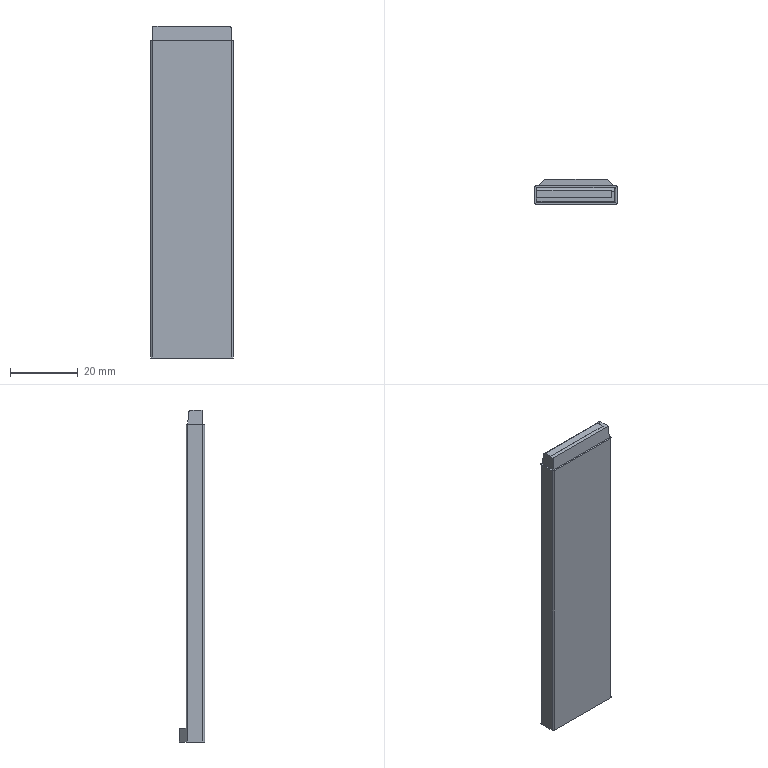Part | Creo | 1 solid | 23 faces | box 24.5 x 7.5 x 98.362 mm | volume 13240 mm3 | plane 18 | cylinder 5 | commonest cylinder face diameters 1 x4 2.01 x1
STEP:
#1=CARTESIAN_POINT('',(0.,0.,0.));
#2=DIRECTION('',(0.,0.,1.));
#3=DIRECTION('',(1.,0.,0.));
#4=AXIS2_PLACEMENT_3D('',#1,#2,#3);
#5=CARTESIAN_POINT('',(-40.598,53.591,40.081));
#6=VERTEX_POINT('',#5);
#7=CARTESIAN_POINT('',(-40.598,53.591,-54.09));
#8=VERTEX_POINT('',#7);
#9=CARTESIAN_POINT('',(-40.598,53.591,40.081));
#10=DIRECTION('',(0.,0.,-1.));
#11=VECTOR('',#10,94.171);
#12=LINE('',#9,#11);
#13=EDGE_CURVE('',#6,#8,#12,.T.);
#14=ORIENTED_EDGE('',*,*,#13,.T.);
#15=CARTESIAN_POINT('',(-40.598,58.091,-54.09));
#16=VERTEX_POINT('',#15);
#17=CARTESIAN_POINT('',(-40.598,53.591,-54.09));
#18=DIRECTION('',(0.,1.,0.));
#19=VECTOR('',#18,4.5);
#20=LINE('',#17,#19);
#21=EDGE_CURVE('',#8,#16,#20,.T.);
#22=ORIENTED_EDGE('',*,*,#21,.T.);
#23=CARTESIAN_POINT('',(-40.598,58.091,40.081));
#24=VERTEX_POINT('',#23);
#25=CARTESIAN_POINT('',(-40.598,58.091,-54.09));
#26=DIRECTION('',(0.,0.,1.));
#27=VECTOR('',#26,94.171);
#28=LINE('',#25,#27);
#29=EDGE_CURVE('',#16,#24,#28,.T.);
#30=ORIENTED_EDGE('',*,*,#29,.T.);
#31=CARTESIAN_POINT('',(-40.598,58.091,40.081));
#32=DIRECTION('',(0.,-1.,0.));
#33=VECTOR('',#32,4.5);
#34=LINE('',#31,#33);
#35=EDGE_CURVE('',#24,#6,#34,.T.);
#36=ORIENTED_EDGE('',*,*,#35,.T.);
#37=EDGE_LOOP('',(#14,#22,#30,#36));
#38=FACE_OUTER_BOUND('',#37,.F.);
#39=CARTESIAN_POINT('',(-40.598,58.591,68.91));
#40=DIRECTION('',(1.,0.,0.));
#41=DIRECTION('',(0.,0.,-1.));
#42=AXIS2_PLACEMENT_3D('',#39,#40,#41);
#43=PLANE('',#42);
#44=ADVANCED_FACE('',(#38),#43,.F.);
#45=CARTESIAN_POINT('',(-40.098,53.091,40.081));
#46=VERTEX_POINT('',#45);
#47=CARTESIAN_POINT('',(-40.098,53.591,40.081));
#48=DIRECTION('',(0.,0.,1.));
#49=DIRECTION('',(-1.,0.,0.));
#50=AXIS2_PLACEMENT_3D('',#47,#48,#49);
#51=CIRCLE('',#50,0.5);
#52=EDGE_CURVE('',#6,#46,#51,.T.);
#53=ORIENTED_EDGE('',*,*,#52,.T.);
#54=CARTESIAN_POINT('',(-40.098,53.091,-54.09));
#55=VERTEX_POINT('',#54);
#56=CARTESIAN_POINT('',(-40.098,53.091,-54.09));
#57=DIRECTION('',(0.,0.,1.));
#58=VECTOR('',#57,94.171);
#59=LINE('',#56,#58);
#60=EDGE_CURVE('',#55,#46,#59,.T.);
#61=ORIENTED_EDGE('',*,*,#60,.F.);
#62=CARTESIAN_POINT('',(-40.098,53.591,-54.09));
#63=DIRECTION('',(0.,0.,-1.));
#64=DIRECTION('',(0.,-1.,0.));
#65=AXIS2_PLACEMENT_3D('',#62,#63,#64);
#66=CIRCLE('',#65,0.5);
#67=EDGE_CURVE('',#55,#8,#66,.T.);
#68=ORIENTED_EDGE('',*,*,#67,.T.);
#69=ORIENTED_EDGE('',*,*,#13,.F.);
#70=EDGE_LOOP('',(#53,#61,#68,#69));
#71=FACE_OUTER_BOUND('',#70,.F.);
#72=CARTESIAN_POINT('',(-40.098,53.591,68.91));
#73=DIRECTION('',(0.,0.,-1.));
#74=DIRECTION('',(-1.,0.,0.));
#75=AXIS2_PLACEMENT_3D('',#72,#73,#74);
#76=CYLINDRICAL_SURFACE('',#75,0.5);
#77=ADVANCED_FACE('',(#71),#76,.T.);
#78=CARTESIAN_POINT('',(-16.598,58.591,40.081));
#79=VERTEX_POINT('',#78);
#80=CARTESIAN_POINT('',(-40.098,58.591,40.081));
#81=VERTEX_POINT('',#80);
#82=CARTESIAN_POINT('',(-16.598,58.591,40.081));
#83=DIRECTION('',(-1.,0.,0.));
#84=VECTOR('',#83,23.5);
#85=LINE('',#82,#84);
#86=EDGE_CURVE('',#79,#81,#85,.T.);
#87=ORIENTED_EDGE('',*,*,#86,.F.);
#88=CARTESIAN_POINT('',(-16.098,58.091,40.081));
#89=VERTEX_POINT('',#88);
#90=CARTESIAN_POINT('',(-16.598,58.091,40.081));
#91=DIRECTION('',(0.,0.,1.));
#92=DIRECTION('',(1.,0.,0.));
#93=AXIS2_PLACEMENT_3D('',#90,#91,#92);
#94=CIRCLE('',#93,0.5);
#95=EDGE_CURVE('',#89,#79,#94,.T.);
#96=ORIENTED_EDGE('',*,*,#95,.F.);
#97=CARTESIAN_POINT('',(-16.098,53.591,40.081));
#98=VERTEX_POINT('',#97);
#99=CARTESIAN_POINT('',(-16.098,53.591,40.081));
#100=DIRECTION('',(0.,1.,0.));
#101=VECTOR('',#100,4.5);
#102=LINE('',#99,#101);
#103=EDGE_CURVE('',#98,#89,#102,.T.);
#104=ORIENTED_EDGE('',*,*,#103,.F.);
#105=CARTESIAN_POINT('',(-16.598,53.091,40.081));
#106=VERTEX_POINT('',#105);
#107=CARTESIAN_POINT('',(-16.598,53.591,40.081));
#108=DIRECTION('',(0.,0.,1.));
#109=DIRECTION('',(0.,-1.,0.));
#110=AXIS2_PLACEMENT_3D('',#107,#108,#109);
#111=CIRCLE('',#110,0.5);
#112=EDGE_CURVE('',#106,#98,#111,.T.);
#113=ORIENTED_EDGE('',*,*,#112,.F.);
#114=CARTESIAN_POINT('',(-40.098,53.091,40.081));
#115=DIRECTION('',(1.,0.,0.));
#116=VECTOR('',#115,23.5);
#117=LINE('',#114,#116);
#118=EDGE_CURVE('',#46,#106,#117,.T.);
#119=ORIENTED_EDGE('',*,*,#118,.F.);
#120=ORIENTED_EDGE('',*,*,#52,.F.);
#121=ORIENTED_EDGE('',*,*,#35,.F.);
#122=CARTESIAN_POINT('',(-40.098,58.091,40.081));
#123=DIRECTION('',(0.,0.,1.));
#124=DIRECTION('',(0.,1.,0.));
#125=AXIS2_PLACEMENT_3D('',#122,#123,#124);
#126=CIRCLE('',#125,0.5);
#127=EDGE_CURVE('',#81,#24,#126,.T.);
#128=ORIENTED_EDGE('',*,*,#127,.F.);
#129=EDGE_LOOP('',(#87,#96,#104,#113,#119,#120,#121,#128));
#130=FACE_OUTER_BOUND('',#129,.F.);
#131=CARTESIAN_POINT('',(-16.598,53.644,40.081));
#132=VERTEX_POINT('',#131);
#133=CARTESIAN_POINT('',(-40.14,53.644,40.081));
#134=VERTEX_POINT('',#133);
#135=CARTESIAN_POINT('',(-16.598,53.644,40.081));
#136=DIRECTION('',(-1.,0.,0.));
#137=VECTOR('',#136,23.542);
#138=LINE('',#135,#137);
#139=EDGE_CURVE('',#132,#134,#138,.T.);
#140=ORIENTED_EDGE('',*,*,#139,.F.);
#141=CARTESIAN_POINT('',(-16.598,58.091,40.081));
#142=VERTEX_POINT('',#141);
#143=CARTESIAN_POINT('',(-16.598,58.091,40.081));
#144=DIRECTION('',(-0.00000001,-1.,0.000000195));
#145=VECTOR('',#144,4.447);
#146=LINE('',#143,#145);
#147=EDGE_CURVE('',#142,#132,#146,.T.);
#148=ORIENTED_EDGE('',*,*,#147,.F.);
#149=CARTESIAN_POINT('',(-40.14,58.091,40.081));
#150=VERTEX_POINT('',#149);
#151=CARTESIAN_POINT('',(-16.598,58.091,40.081));
#152=DIRECTION('',(-1.,0.,0.));
#153=VECTOR('',#152,23.542);
#154=LINE('',#151,#153);
#155=EDGE_CURVE('',#142,#150,#154,.T.);
#156=ORIENTED_EDGE('',*,*,#155,.T.);
#157=CARTESIAN_POINT('',(-40.14,58.091,40.081));
#158=DIRECTION('',(0.00000001,-1.,0.000000195));
#159=VECTOR('',#158,4.447);
#160=LINE('',#157,#159);
#161=EDGE_CURVE('',#150,#134,#160,.T.);
#162=ORIENTED_EDGE('',*,*,#161,.T.);
#163=EDGE_LOOP('',(#140,#148,#156,#162));
#164=FACE_BOUND('',#163,.F.);
#165=CARTESIAN_POINT('',(-17.817,-88.35,40.081));
#166=DIRECTION('',(0.,0.,1.));
#167=DIRECTION('',(-1.,0.,0.));
#168=AXIS2_PLACEMENT_3D('',#165,#166,#167);
#169=PLANE('',#168);
#170=ADVANCED_FACE('',(#130,#164),#169,.T.);
#171=CARTESIAN_POINT('',(-40.098,58.591,-54.09));
#172=VERTEX_POINT('',#171);
#173=CARTESIAN_POINT('',(-40.098,58.591,40.081));
#174=DIRECTION('',(0.,0.,-1.));
#175=VECTOR('',#174,94.171);
#176=LINE('',#173,#175);
#177=EDGE_CURVE('',#81,#172,#176,.T.);
#178=ORIENTED_EDGE('',*,*,#177,.T.);
#179=CARTESIAN_POINT('',(-39.598,58.591,-54.09));
#180=VERTEX_POINT('',#179);
#181=CARTESIAN_POINT('',(-40.098,58.591,-54.09));
#182=DIRECTION('',(1.,0.,0.));
#183=VECTOR('',#182,0.5);
#184=LINE('',#181,#183);
#185=EDGE_CURVE('',#172,#180,#184,.T.);
#186=ORIENTED_EDGE('',*,*,#185,.T.);
#187=CARTESIAN_POINT('',(-39.598,58.591,-50.09));
#188=VERTEX_POINT('',#187);
#189=CARTESIAN_POINT('',(-39.598,58.591,-54.09));
#190=DIRECTION('',(0.,0.,1.));
#191=VECTOR('',#190,4.);
#192=LINE('',#189,#191);
#193=EDGE_CURVE('',#180,#188,#192,.T.);
#194=ORIENTED_EDGE('',*,*,#193,.T.);
#195=CARTESIAN_POINT('',(-17.098,58.591,-50.09));
#196=VERTEX_POINT('',#195);
#197=CARTESIAN_POINT('',(-39.598,58.591,-50.09));
#198=DIRECTION('',(1.,0.,0.));
#199=VECTOR('',#198,22.5);
#200=LINE('',#197,#199);
#201=EDGE_CURVE('',#188,#196,#200,.T.);
#202=ORIENTED_EDGE('',*,*,#201,.T.);
#203=CARTESIAN_POINT('',(-17.098,58.591,-54.09));
#204=VERTEX_POINT('',#203);
#205=CARTESIAN_POINT('',(-17.098,58.591,-50.09));
#206=DIRECTION('',(0.,0.,-1.));
#207=VECTOR('',#206,4.);
#208=LINE('',#205,#207);
#209=EDGE_CURVE('',#196,#204,#208,.T.);
#210=ORIENTED_EDGE('',*,*,#209,.T.);
#211=CARTESIAN_POINT('',(-16.598,58.591,-54.09));
#212=VERTEX_POINT('',#211);
#213=CARTESIAN_POINT('',(-17.098,58.591,-54.09));
#214=DIRECTION('',(1.,0.,0.));
#215=VECTOR('',#214,0.5);
#216=LINE('',#213,#215);
#217=EDGE_CURVE('',#204,#212,#216,.T.);
#218=ORIENTED_EDGE('',*,*,#217,.T.);
#219=CARTESIAN_POINT('',(-16.598,58.591,-54.09));
#220=DIRECTION('',(0.,0.,1.));
#221=VECTOR('',#220,94.171);
#222=LINE('',#219,#221);
#223=EDGE_CURVE('',#212,#79,#222,.T.);
#224=ORIENTED_EDGE('',*,*,#223,.T.);
#225=ORIENTED_EDGE('',*,*,#86,.T.);
#226=EDGE_LOOP('',(#178,#186,#194,#202,#210,#218,#224,#225));
#227=FACE_OUTER_BOUND('',#226,.F.);
#228=CARTESIAN_POINT('',(-16.098,58.591,68.91));
#229=DIRECTION('',(0.,-1.,0.));
#230=DIRECTION('',(0.,0.,-1.));
#231=AXIS2_PLACEMENT_3D('',#228,#229,#230);
#232=PLANE('',#231);
#233=ADVANCED_FACE('',(#227),#232,.F.);
#234=ORIENTED_EDGE('',*,*,#127,.T.);
#235=ORIENTED_EDGE('',*,*,#29,.F.);
#236=CARTESIAN_POINT('',(-40.098,58.091,-54.09));
#237=DIRECTION('',(0.,0.,-1.));
#238=DIRECTION('',(-1.,0.,0.));
#239=AXIS2_PLACEMENT_3D('',#236,#237,#238);
#240=CIRCLE('',#239,0.5);
#241=EDGE_CURVE('',#16,#172,#240,.T.);
#242=ORIENTED_EDGE('',*,*,#241,.T.);
#243=ORIENTED_EDGE('',*,*,#177,.F.);
#244=EDGE_LOOP('',(#234,#235,#242,#243));
#245=FACE_OUTER_BOUND('',#244,.F.);
#246=CARTESIAN_POINT('',(-40.098,58.091,68.91));
#247=DIRECTION('',(0.,0.,-1.));
#248=DIRECTION('',(-1.,0.,0.));
#249=AXIS2_PLACEMENT_3D('',#246,#247,#248);
#250=CYLINDRICAL_SURFACE('',#249,0.5);
#251=ADVANCED_FACE('',(#245),#250,.T.);
#252=CARTESIAN_POINT('',(-37.598,60.591,-54.09));
#253=VERTEX_POINT('',#252);
#254=CARTESIAN_POINT('',(-19.098,60.591,-54.09));
#255=VERTEX_POINT('',#254);
#256=CARTESIAN_POINT('',(-37.598,60.591,-54.09));
#257=DIRECTION('',(1.,0.,0.));
#258=VECTOR('',#257,18.5);
#259=LINE('',#256,#258);
#260=EDGE_CURVE('',#253,#255,#259,.T.);
#261=ORIENTED_EDGE('',*,*,#260,.F.);
#262=CARTESIAN_POINT('',(-39.598,58.591,-54.09));
#263=DIRECTION('',(0.7071,0.7071,0.));
#264=VECTOR('',#263,2.828);
#265=LINE('',#262,#264);
#266=EDGE_CURVE('',#180,#253,#265,.T.);
#267=ORIENTED_EDGE('',*,*,#266,.F.);
#268=ORIENTED_EDGE('',*,*,#185,.F.);
#269=ORIENTED_EDGE('',*,*,#241,.F.);
#270=ORIENTED_EDGE('',*,*,#21,.F.);
#271=ORIENTED_EDGE('',*,*,#67,.F.);
#272=CARTESIAN_POINT('',(-16.598,53.091,-54.09));
#273=VERTEX_POINT('',#272);
#274=CARTESIAN_POINT('',(-16.598,53.091,-54.09));
#275=DIRECTION('',(-1.,0.,0.));
#276=VECTOR('',#275,23.5);
#277=LINE('',#274,#276);
#278=EDGE_CURVE('',#273,#55,#277,.T.);
#279=ORIENTED_EDGE('',*,*,#278,.F.);
#280=CARTESIAN_POINT('',(-16.098,53.591,-54.09));
#281=VERTEX_POINT('',#280);
#282=CARTESIAN_POINT('',(-16.598,53.591,-54.09));
#283=DIRECTION('',(0.,0.,-1.));
#284=DIRECTION('',(1.,0.,0.));
#285=AXIS2_PLACEMENT_3D('',#282,#283,#284);
#286=CIRCLE('',#285,0.5);
#287=EDGE_CURVE('',#281,#273,#286,.T.);
#288=ORIENTED_EDGE('',*,*,#287,.F.);
#289=CARTESIAN_POINT('',(-16.098,58.091,-54.09));
#290=VERTEX_POINT('',#289);
#291=CARTESIAN_POINT('',(-16.098,58.091,-54.09));
#292=DIRECTION('',(0.,-1.,0.));
#293=VECTOR('',#292,4.5);
#294=LINE('',#291,#293);
#295=EDGE_CURVE('',#290,#281,#294,.T.);
#296=ORIENTED_EDGE('',*,*,#295,.F.);
#297=CARTESIAN_POINT('',(-16.598,58.091,-54.09));
#298=DIRECTION('',(0.,0.,-1.));
#299=DIRECTION('',(0.,1.,0.));
#300=AXIS2_PLACEMENT_3D('',#297,#298,#299);
#301=CIRCLE('',#300,0.5);
#302=EDGE_CURVE('',#212,#290,#301,.T.);
#303=ORIENTED_EDGE('',*,*,#302,.F.);
#304=ORIENTED_EDGE('',*,*,#217,.F.);
#305=CARTESIAN_POINT('',(-19.098,60.591,-54.09));
#306=DIRECTION('',(0.7071,-0.7071,0.));
#307=VECTOR('',#306,2.828);
#308=LINE('',#305,#307);
#309=EDGE_CURVE('',#255,#204,#308,.T.);
#310=ORIENTED_EDGE('',*,*,#309,.F.);
#311=EDGE_LOOP('',(#261,#267,#268,#269,#270,#271,#279,#288,#296,#303,#304,#310));
#312=FACE_OUTER_BOUND('',#311,.F.);
#313=CARTESIAN_POINT('',(0.,0.,-54.09));
#314=DIRECTION('',(0.,0.,-1.));
#315=DIRECTION('',(-1.,0.,0.));
#316=AXIS2_PLACEMENT_3D('',#313,#314,#315);
#317=PLANE('',#316);
#318=ADVANCED_FACE('',(#312),#317,.T.);
#319=CARTESIAN_POINT('',(-19.098,60.591,-50.09));
#320=VERTEX_POINT('',#319);
#321=CARTESIAN_POINT('',(-37.598,60.591,-50.09));
#322=VERTEX_POINT('',#321);
#323=CARTESIAN_POINT('',(-19.098,60.591,-50.09));
#324=DIRECTION('',(-1.,0.,0.));
#325=VECTOR('',#324,18.5);
#326=LINE('',#323,#325);
#327=EDGE_CURVE('',#320,#322,#326,.T.);
#328=ORIENTED_EDGE('',*,*,#327,.T.);
#329=CARTESIAN_POINT('',(-37.598,60.591,-50.09));
#330=DIRECTION('',(0.,0.,-1.));
#331=VECTOR('',#330,4.);
#332=LINE('',#329,#331);
#333=EDGE_CURVE('',#322,#253,#332,.T.);
#334=ORIENTED_EDGE('',*,*,#333,.T.);
#335=ORIENTED_EDGE('',*,*,#260,.T.);
#336=CARTESIAN_POINT('',(-19.098,60.591,-54.09));
#337=DIRECTION('',(0.,0.,1.));
#338=VECTOR('',#337,4.);
#339=LINE('',#336,#338);
#340=EDGE_CURVE('',#255,#320,#339,.T.);
#341=ORIENTED_EDGE('',*,*,#340,.T.);
#342=EDGE_LOOP('',(#328,#334,#335,#341));
#343=FACE_OUTER_BOUND('',#342,.F.);
#344=CARTESIAN_POINT('',(-28.348,60.591,-44.09));
#345=DIRECTION('',(0.,1.,0.));
#346=DIRECTION('',(0.,0.,1.));
#347=AXIS2_PLACEMENT_3D('',#344,#345,#346);
#348=PLANE('',#347);
#349=ADVANCED_FACE('',(#343),#348,.T.);
#350=ORIENTED_EDGE('',*,*,#201,.F.);
#351=CARTESIAN_POINT('',(-37.598,60.591,-50.09));
#352=DIRECTION('',(-0.7071,-0.7071,0.));
#353=VECTOR('',#352,2.828);
#354=LINE('',#351,#353);
#355=EDGE_CURVE('',#322,#188,#354,.T.);
#356=ORIENTED_EDGE('',*,*,#355,.F.);
#357=ORIENTED_EDGE('',*,*,#327,.F.);
#358=CARTESIAN_POINT('',(-17.098,58.591,-50.09));
#359=DIRECTION('',(-0.7071,0.7071,0.));
#360=VECTOR('',#359,2.828);
#361=LINE('',#358,#360);
#362=EDGE_CURVE('',#196,#320,#361,.T.);
#363=ORIENTED_EDGE('',*,*,#362,.F.);
#364=EDGE_LOOP('',(#350,#356,#357,#363));
#365=FACE_OUTER_BOUND('',#364,.F.);
#366=CARTESIAN_POINT('',(-28.348,59.091,-50.09));
#367=DIRECTION('',(0.,0.,1.));
#368=DIRECTION('',(1.,0.,0.));
#369=AXIS2_PLACEMENT_3D('',#366,#367,#368);
#370=PLANE('',#369);
#371=ADVANCED_FACE('',(#365),#370,.T.);
#372=ORIENTED_EDGE('',*,*,#266,.T.);
#373=ORIENTED_EDGE('',*,*,#333,.F.);
#374=ORIENTED_EDGE('',*,*,#355,.T.);
#375=ORIENTED_EDGE('',*,*,#193,.F.);
#376=EDGE_LOOP('',(#372,#373,#374,#375));
#377=FACE_OUTER_BOUND('',#376,.F.);
#378=CARTESIAN_POINT('',(-37.598,60.591,-44.09));
#379=DIRECTION('',(0.7071,-0.7071,0.));
#380=DIRECTION('',(0.,0.,1.));
#381=AXIS2_PLACEMENT_3D('',#378,#379,#380);
#382=PLANE('',#381);
#383=ADVANCED_FACE('',(#377),#382,.F.);
#384=ORIENTED_EDGE('',*,*,#309,.T.);
#385=ORIENTED_EDGE('',*,*,#209,.F.);
#386=ORIENTED_EDGE('',*,*,#362,.T.);
#387=ORIENTED_EDGE('',*,*,#340,.F.);
#388=EDGE_LOOP('',(#384,#385,#386,#387));
#389=FACE_OUTER_BOUND('',#388,.F.);
#390=CARTESIAN_POINT('',(-17.098,58.591,-44.09));
#391=DIRECTION('',(-0.7071,-0.7071,0.));
#392=DIRECTION('',(0.,0.,1.));
#393=AXIS2_PLACEMENT_3D('',#390,#391,#392);
#394=PLANE('',#393);
#395=ADVANCED_FACE('',(#389),#394,.F.);
#396=CARTESIAN_POINT('',(-16.598,53.091,40.081));
#397=DIRECTION('',(0.,0.,-1.));
#398=VECTOR('',#397,94.171);
#399=LINE('',#396,#398);
#400=EDGE_CURVE('',#106,#273,#399,.T.);
#401=ORIENTED_EDGE('',*,*,#400,.T.);
#402=ORIENTED_EDGE('',*,*,#278,.T.);
#403=ORIENTED_EDGE('',*,*,#60,.T.);
#404=ORIENTED_EDGE('',*,*,#118,.T.);
#405=EDGE_LOOP('',(#401,#402,#403,#404));
#406=FACE_OUTER_BOUND('',#405,.F.);
#407=CARTESIAN_POINT('',(-40.598,53.091,68.91));
#408=DIRECTION('',(0.,1.,0.));
#409=DIRECTION('',(0.,0.,1.));
#410=AXIS2_PLACEMENT_3D('',#407,#408,#409);
#411=PLANE('',#410);
#412=ADVANCED_FACE('',(#406),#411,.F.);
#413=ORIENTED_EDGE('',*,*,#112,.T.);
#414=CARTESIAN_POINT('',(-16.098,53.591,-54.09));
#415=DIRECTION('',(0.,0.,1.));
#416=VECTOR('',#415,94.171);
#417=LINE('',#414,#416);
#418=EDGE_CURVE('',#281,#98,#417,.T.);
#419=ORIENTED_EDGE('',*,*,#418,.F.);
#420=ORIENTED_EDGE('',*,*,#287,.T.);
#421=ORIENTED_EDGE('',*,*,#400,.F.);
#422=EDGE_LOOP('',(#413,#419,#420,#421));
#423=FACE_OUTER_BOUND('',#422,.F.);
#424=CARTESIAN_POINT('',(-16.598,53.591,68.91));
#425=DIRECTION('',(0.,0.,-1.));
#426=DIRECTION('',(-1.,0.,0.));
#427=AXIS2_PLACEMENT_3D('',#424,#425,#426);
#428=CYLINDRICAL_SURFACE('',#427,0.5);
#429=ADVANCED_FACE('',(#423),#428,.T.);
#430=CARTESIAN_POINT('',(-16.098,58.091,40.081));
#431=DIRECTION('',(0.,0.,-1.));
#432=VECTOR('',#431,94.171);
#433=LINE('',#430,#432);
#434=EDGE_CURVE('',#89,#290,#433,.T.);
#435=ORIENTED_EDGE('',*,*,#434,.T.);
#436=ORIENTED_EDGE('',*,*,#295,.T.);
#437=ORIENTED_EDGE('',*,*,#418,.T.);
#438=ORIENTED_EDGE('',*,*,#103,.T.);
#439=EDGE_LOOP('',(#435,#436,#437,#438));
#440=FACE_OUTER_BOUND('',#439,.F.);
#441=CARTESIAN_POINT('',(-16.098,53.091,68.91));
#442=DIRECTION('',(-1.,0.,0.));
#443=DIRECTION('',(0.,0.,1.));
#444=AXIS2_PLACEMENT_3D('',#441,#442,#443);
#445=PLANE('',#444);
#446=ADVANCED_FACE('',(#440),#445,.F.);
#447=ORIENTED_EDGE('',*,*,#95,.T.);
#448=ORIENTED_EDGE('',*,*,#223,.F.);
#449=ORIENTED_EDGE('',*,*,#302,.T.);
#450=ORIENTED_EDGE('',*,*,#434,.F.);
#451=EDGE_LOOP('',(#447,#448,#449,#450));
#452=FACE_OUTER_BOUND('',#451,.F.);
#453=CARTESIAN_POINT('',(-16.598,58.091,68.91));
#454=DIRECTION('',(0.,0.,-1.));
#455=DIRECTION('',(-1.,0.,0.));
#456=AXIS2_PLACEMENT_3D('',#453,#454,#455);
#457=CYLINDRICAL_SURFACE('',#456,0.5);
#458=ADVANCED_FACE('',(#452),#457,.T.);
#459=CARTESIAN_POINT('',(-16.818,53.864,44.272));
#460=VERTEX_POINT('',#459);
#461=CARTESIAN_POINT('',(-16.818,53.864,44.272));
#462=DIRECTION('',(0.05226,-0.05226,-0.9973));
#463=VECTOR('',#462,4.202);
#464=LINE('',#461,#463);
#465=EDGE_CURVE('',#460,#132,#464,.T.);
#466=ORIENTED_EDGE('',*,*,#465,.T.);
#467=ORIENTED_EDGE('',*,*,#139,.T.);
#468=CARTESIAN_POINT('',(-39.92,53.864,44.272));
#469=VERTEX_POINT('',#468);
#470=CARTESIAN_POINT('',(-39.92,53.864,44.272));
#471=DIRECTION('',(-0.05226,-0.05226,-0.9973));
#472=VECTOR('',#471,4.202);
#473=LINE('',#470,#472);
#474=EDGE_CURVE('',#469,#134,#473,.T.);
#475=ORIENTED_EDGE('',*,*,#474,.F.);
#476=CARTESIAN_POINT('',(-39.92,53.864,44.272));
#477=DIRECTION('',(1.,0.,0.));
#478=VECTOR('',#477,23.102);
#479=LINE('',#476,#478);
#480=EDGE_CURVE('',#469,#460,#479,.T.);
#481=ORIENTED_EDGE('',*,*,#480,.T.);
#482=EDGE_LOOP('',(#466,#467,#475,#481));
#483=FACE_OUTER_BOUND('',#482,.F.);
#484=CARTESIAN_POINT('',(-42.536,53.858,44.151));
#485=DIRECTION('',(0.,-0.9986,0.05234));
#486=DIRECTION('',(1.,0.,0.));
#487=AXIS2_PLACEMENT_3D('',#484,#485,#486);
#488=PLANE('',#487);
#489=ADVANCED_FACE('',(#483),#488,.T.);
#490=CARTESIAN_POINT('',(-16.768,57.925,43.318));
#491=VERTEX_POINT('',#490);
#492=CARTESIAN_POINT('',(-16.768,57.925,43.318));
#493=DIRECTION('',(0.05227,0.05114,-0.9973));
#494=VECTOR('',#493,3.246);
#495=LINE('',#492,#494);
#496=EDGE_CURVE('',#491,#142,#495,.T.);
#497=ORIENTED_EDGE('',*,*,#496,.T.);
#498=ORIENTED_EDGE('',*,*,#147,.T.);
#499=ORIENTED_EDGE('',*,*,#465,.F.);
#500=CARTESIAN_POINT('',(-16.818,56.921,44.272));
#501=VERTEX_POINT('',#500);
#502=CARTESIAN_POINT('',(-16.818,53.864,44.272));
#503=DIRECTION('',(0.,1.,0.));
#504=VECTOR('',#503,3.057);
#505=LINE('',#502,#504);
#506=EDGE_CURVE('',#460,#501,#505,.T.);
#507=ORIENTED_EDGE('',*,*,#506,.T.);
#508=CARTESIAN_POINT('',(-16.818,56.921,44.272));
#509=CARTESIAN_POINT('',(-16.818,57.08,44.272));
#510=CARTESIAN_POINT('',(-16.814,57.335,44.205));
#511=CARTESIAN_POINT('',(-16.804,57.627,44.009));
#512=CARTESIAN_POINT('',(-16.789,57.837,43.728));
#513=CARTESIAN_POINT('',(-16.776,57.917,43.477));
#514=B_SPLINE_CURVE_WITH_KNOTS('',3,(#508,#509,#510,#511,#512,#513,#490),.UNSPECIFIED.,.F.,.F.,(4,1,1,1,4),(0.,0.25,0.5,0.75,1.),.UNSPECIFIED.);
#515=EDGE_CURVE('',#501,#491,#514,.T.);
#516=ORIENTED_EDGE('',*,*,#515,.T.);
#517=EDGE_LOOP('',(#497,#498,#499,#507,#516));
#518=FACE_OUTER_BOUND('',#517,.F.);
#519=CARTESIAN_POINT('',(-16.811,-91.965,44.151));
#520=DIRECTION('',(0.9986,0.,0.05234));
#521=DIRECTION('',(0.,1.,0.));
#522=AXIS2_PLACEMENT_3D('',#519,#520,#521);
#523=PLANE('',#522);
#524=ADVANCED_FACE('',(#518),#523,.T.);
#525=CARTESIAN_POINT('',(-39.97,57.925,43.318));
#526=VERTEX_POINT('',#525);
#527=CARTESIAN_POINT('',(-16.768,57.925,43.318));
#528=DIRECTION('',(-1.,0.,0.));
#529=VECTOR('',#528,23.202);
#530=LINE('',#527,#529);
#531=EDGE_CURVE('',#491,#526,#530,.T.);
#532=ORIENTED_EDGE('',*,*,#531,.T.);
#533=CARTESIAN_POINT('',(-40.14,58.091,40.081));
#534=DIRECTION('',(0.05227,-0.05114,0.9973));
#535=VECTOR('',#534,3.246);
#536=LINE('',#533,#535);
#537=EDGE_CURVE('',#150,#526,#536,.T.);
#538=ORIENTED_EDGE('',*,*,#537,.F.);
#539=ORIENTED_EDGE('',*,*,#155,.F.);
#540=ORIENTED_EDGE('',*,*,#496,.F.);
#541=EDGE_LOOP('',(#532,#538,#539,#540));
#542=FACE_OUTER_BOUND('',#541,.F.);
#543=CARTESIAN_POINT('',(-42.536,57.882,44.151));
#544=DIRECTION('',(0.,0.9987,0.05121));
#545=DIRECTION('',(-1.,0.,0.));
#546=AXIS2_PLACEMENT_3D('',#543,#544,#545);
#547=PLANE('',#546);
#548=ADVANCED_FACE('',(#542),#547,.T.);
#549=CARTESIAN_POINT('',(-17.902,56.921,44.272));
#550=VERTEX_POINT('',#549);
#551=CARTESIAN_POINT('',(-17.902,57.202,44.231));
#552=VERTEX_POINT('',#551);
#553=CARTESIAN_POINT('',(-17.902,56.921,43.267));
#554=DIRECTION('',(-1.,0.,0.));
#555=DIRECTION('',(0.,0.,1.));
#556=AXIS2_PLACEMENT_3D('',#553,#554,#555);
#557=CIRCLE('',#556,1.005);
#558=EDGE_CURVE('',#550,#552,#557,.T.);
#559=ORIENTED_EDGE('',*,*,#558,.T.);
#560=CARTESIAN_POINT('',(-39.922,57.202,44.231));
#561=VERTEX_POINT('',#560);
#562=CARTESIAN_POINT('',(-39.922,57.202,44.231));
#563=DIRECTION('',(1.,0.,0.));
#564=VECTOR('',#563,22.02);
#565=LINE('',#562,#564);
#566=EDGE_CURVE('',#561,#552,#565,.T.);
#567=ORIENTED_EDGE('',*,*,#566,.F.);
#568=CARTESIAN_POINT('',(-39.926,57.431,44.165));
#569=CARTESIAN_POINT('',(-39.939,57.747,43.92));
#570=CARTESIAN_POINT('',(-39.958,57.913,43.556));
#571=CARTESIAN_POINT('',(-39.97,57.925,43.318));
#572=B_SPLINE_CURVE_WITH_KNOTS('',3,(#560,#568,#569,#570,#571),.UNSPECIFIED.,.F.,.F.,(4,1,4),(0.,0.5,1.),.UNSPECIFIED.);
#573=EDGE_CURVE('',#561,#526,#572,.T.);
#574=ORIENTED_EDGE('',*,*,#573,.T.);
#575=ORIENTED_EDGE('',*,*,#531,.F.);
#576=ORIENTED_EDGE('',*,*,#515,.F.);
#577=CARTESIAN_POINT('',(-17.902,56.921,44.272));
#578=DIRECTION('',(1.,0.,0.));
#579=VECTOR('',#578,1.085);
#580=LINE('',#577,#579);
#581=EDGE_CURVE('',#550,#501,#580,.T.);
#582=ORIENTED_EDGE('',*,*,#581,.F.);
#583=EDGE_LOOP('',(#559,#567,#574,#575,#576,#582));
#584=FACE_OUTER_BOUND('',#583,.F.);
#585=CARTESIAN_POINT('',(-16.811,56.921,43.267));
#586=DIRECTION('',(-1.,0.,0.));
#587=DIRECTION('',(0.,0.,1.));
#588=AXIS2_PLACEMENT_3D('',#585,#586,#587);
#589=CYLINDRICAL_SURFACE('',#588,1.005);
#590=ADVANCED_FACE('',(#584),#589,.T.);
#591=ORIENTED_EDGE('',*,*,#558,.F.);
#592=CARTESIAN_POINT('',(-17.902,54.948,44.272));
#593=VERTEX_POINT('',#592);
#594=CARTESIAN_POINT('',(-17.902,56.921,44.272));
#595=DIRECTION('',(0.,-1.,0.));
#596=VECTOR('',#595,1.973);
#597=LINE('',#594,#596);
#598=EDGE_CURVE('',#550,#593,#597,.T.);
#599=ORIENTED_EDGE('',*,*,#598,.T.);
#600=CARTESIAN_POINT('',(-17.902,54.948,44.231));
#601=VERTEX_POINT('',#600);
#602=CARTESIAN_POINT('',(-17.902,54.948,44.272));
#603=DIRECTION('',(0.,0.,-1.));
#604=VECTOR('',#603,0.04);
#605=LINE('',#602,#604);
#606=EDGE_CURVE('',#593,#601,#605,.T.);
#607=ORIENTED_EDGE('',*,*,#606,.T.);
#608=CARTESIAN_POINT('',(-17.902,57.202,44.231));
#609=DIRECTION('',(0.,-1.,0.));
#610=VECTOR('',#609,2.253);
#611=LINE('',#608,#610);
#612=EDGE_CURVE('',#552,#601,#611,.T.);
#613=ORIENTED_EDGE('',*,*,#612,.F.);
#614=EDGE_LOOP('',(#591,#599,#607,#613));
#615=FACE_OUTER_BOUND('',#614,.F.);
#616=CARTESIAN_POINT('',(-17.902,56.924,45.151));
#617=DIRECTION('',(1.,0.,0.));
#618=DIRECTION('',(0.,0.,-1.));
#619=AXIS2_PLACEMENT_3D('',#616,#617,#618);
#620=PLANE('',#619);
#621=ADVANCED_FACE('',(#615),#620,.F.);
#622=ORIENTED_EDGE('',*,*,#598,.F.);
#623=ORIENTED_EDGE('',*,*,#581,.T.);
#624=ORIENTED_EDGE('',*,*,#506,.F.);
#625=ORIENTED_EDGE('',*,*,#480,.F.);
#626=CARTESIAN_POINT('',(-39.92,54.948,44.272));
#627=VERTEX_POINT('',#626);
#628=CARTESIAN_POINT('',(-39.92,54.948,44.272));
#629=DIRECTION('',(0.,-1.,0.));
#630=VECTOR('',#629,1.085);
#631=LINE('',#628,#630);
#632=EDGE_CURVE('',#627,#469,#631,.T.);
#633=ORIENTED_EDGE('',*,*,#632,.F.);
#634=CARTESIAN_POINT('',(-17.902,54.948,44.272));
#635=DIRECTION('',(-1.,0.,0.));
#636=VECTOR('',#635,22.018);
#637=LINE('',#634,#636);
#638=EDGE_CURVE('',#593,#627,#637,.T.);
#639=ORIENTED_EDGE('',*,*,#638,.F.);
#640=EDGE_LOOP('',(#622,#623,#624,#625,#633,#639));
#641=FACE_OUTER_BOUND('',#640,.F.);
#642=CARTESIAN_POINT('',(-16.811,57.877,44.272));
#643=DIRECTION('',(0.,0.,1.));
#644=DIRECTION('',(0.,1.,0.));
#645=AXIS2_PLACEMENT_3D('',#642,#643,#644);
#646=PLANE('',#645);
#647=ADVANCED_FACE('',(#641),#646,.T.);
#648=CARTESIAN_POINT('',(-39.922,54.948,44.231));
#649=VERTEX_POINT('',#648);
#650=CARTESIAN_POINT('',(-39.92,54.948,44.272));
#651=DIRECTION('',(-0.05234,0.,-0.9986));
#652=VECTOR('',#651,0.04005);
#653=LINE('',#650,#652);
#654=EDGE_CURVE('',#627,#649,#653,.T.);
#655=ORIENTED_EDGE('',*,*,#654,.F.);
#656=ORIENTED_EDGE('',*,*,#632,.T.);
#657=ORIENTED_EDGE('',*,*,#474,.T.);
#658=ORIENTED_EDGE('',*,*,#161,.F.);
#659=ORIENTED_EDGE('',*,*,#537,.T.);
#660=ORIENTED_EDGE('',*,*,#573,.F.);
#661=CARTESIAN_POINT('',(-39.922,54.948,44.231));
#662=DIRECTION('',(0.,1.,0.));
#663=VECTOR('',#662,2.253);
#664=LINE('',#661,#663);
#665=EDGE_CURVE('',#649,#561,#664,.T.);
#666=ORIENTED_EDGE('',*,*,#665,.F.);
#667=EDGE_LOOP('',(#655,#656,#657,#658,#659,#660,#666));
#668=FACE_OUTER_BOUND('',#667,.F.);
#669=CARTESIAN_POINT('',(-39.926,-91.965,44.151));
#670=DIRECTION('',(0.9986,0.,-0.05234));
#671=DIRECTION('',(0.,1.,0.));
#672=AXIS2_PLACEMENT_3D('',#669,#670,#671);
#673=PLANE('',#672);
#674=ADVANCED_FACE('',(#668),#673,.F.);
#675=ORIENTED_EDGE('',*,*,#638,.T.);
#676=ORIENTED_EDGE('',*,*,#654,.T.);
#677=CARTESIAN_POINT('',(-17.902,54.948,44.231));
#678=DIRECTION('',(-1.,0.,0.));
#679=VECTOR('',#678,22.02);
#680=LINE('',#677,#679);
#681=EDGE_CURVE('',#601,#649,#680,.T.);
#682=ORIENTED_EDGE('',*,*,#681,.F.);
#683=ORIENTED_EDGE('',*,*,#606,.F.);
#684=EDGE_LOOP('',(#675,#676,#682,#683));
#685=FACE_OUTER_BOUND('',#684,.F.);
#686=CARTESIAN_POINT('',(-17.852,54.948,45.151));
#687=DIRECTION('',(0.,-1.,0.));
#688=DIRECTION('',(0.,0.,-1.));
#689=AXIS2_PLACEMENT_3D('',#686,#687,#688);
#690=PLANE('',#689);
#691=ADVANCED_FACE('',(#685),#690,.F.);
#692=ORIENTED_EDGE('',*,*,#665,.T.);
#693=ORIENTED_EDGE('',*,*,#566,.T.);
#694=ORIENTED_EDGE('',*,*,#612,.T.);
#695=ORIENTED_EDGE('',*,*,#681,.T.);
#696=EDGE_LOOP('',(#692,#693,#694,#695));
#697=FACE_OUTER_BOUND('',#696,.F.);
#698=CARTESIAN_POINT('',(-16.811,57.877,44.231));
#699=DIRECTION('',(0.,0.,1.));
#700=DIRECTION('',(0.,1.,0.));
#701=AXIS2_PLACEMENT_3D('',#698,#699,#700);
#702=PLANE('',#701);
#703=ADVANCED_FACE('',(#697),#702,.T.);
#704=CLOSED_SHELL('',(#44,#77,#170,#233,#251,#318,#349,#371,#383,#395,#412,#429,#446,#458,#489,#524,#548,#590,#621,#647,#674,#691,#703));
#705=MANIFOLD_SOLID_BREP('',#704);
#706=(LENGTH_UNIT()NAMED_UNIT(*)SI_UNIT(.MILLI.,.METRE.));
#707=UNCERTAINTY_MEASURE_WITH_UNIT(LENGTH_MEASURE(0.01016),#706,'','');
#708=(NAMED_UNIT(*)PLANE_ANGLE_UNIT()SI_UNIT($,.RADIAN.));
#709=PLANE_ANGLE_MEASURE_WITH_UNIT(PLANE_ANGLE_MEASURE(0.01745),#708);
#710=(CONVERSION_BASED_UNIT('DEGREE',#709)NAMED_UNIT(*)PLANE_ANGLE_UNIT());
#711=(NAMED_UNIT(*)SI_UNIT($,.STERADIAN.)SOLID_ANGLE_UNIT());
#712=(GEOMETRIC_REPRESENTATION_CONTEXT(3)GLOBAL_UNCERTAINTY_ASSIGNED_CONTEXT((#707))GLOBAL_UNIT_ASSIGNED_CONTEXT((#706,#710,#711))REPRESENTATION_CONTEXT('',''));
#713=ADVANCED_BREP_SHAPE_REPRESENTATION('',(#4,#705),#712);